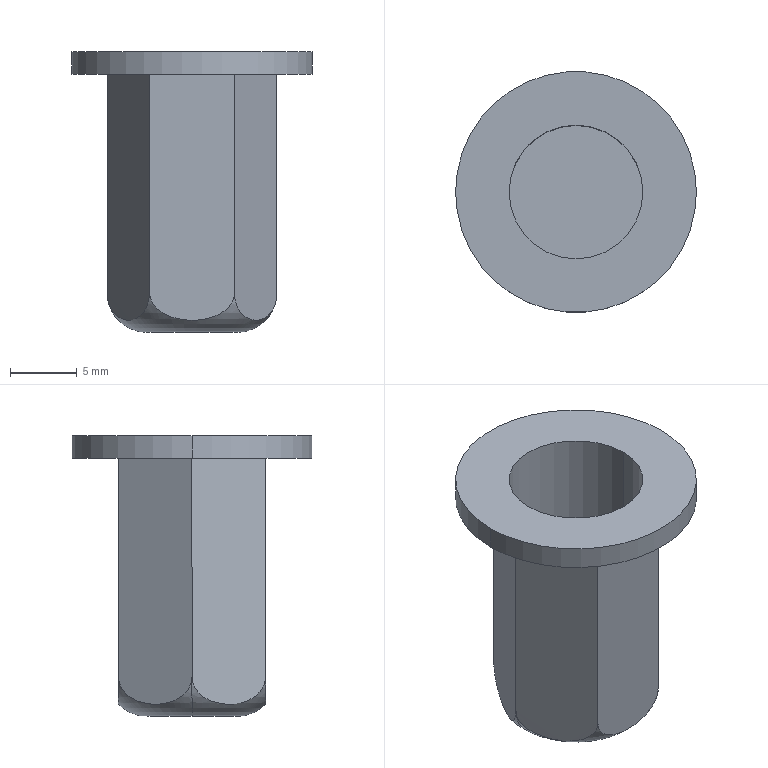Part | SolidWorks | features BaseBody 1 | 1 solid | 16 faces | box 18 x 18 x 21 mm | volume 1010 mm3 | plane 10 | cylinder 4 | torus 2 | commonest cylinder face diameters 10 x2 18 x2
STEP:
#1=CARTESIAN_POINT('',(5.,0.,-16.3));
#2=VERTEX_POINT('',#1);
#3=CARTESIAN_POINT('',(-5.,0.,-16.3));
#4=VERTEX_POINT('',#3);
#5=CARTESIAN_POINT('',(0.,0.,-16.3));
#6=DIRECTION('',(0.,0.,1.));
#7=DIRECTION('',(1.,0.,0.));
#8=AXIS2_PLACEMENT_3D('',#5,#6,#7);
#9=CIRCLE('',#8,5.);
#10=EDGE_CURVE('',#2,#4,#9,.T.);
#11=ORIENTED_EDGE('',*,*,#10,.T.);
#12=CARTESIAN_POINT('',(0.,0.,-16.3));
#13=DIRECTION('',(0.,0.,1.));
#14=DIRECTION('',(1.,0.,0.));
#15=AXIS2_PLACEMENT_3D('',#12,#13,#14);
#16=CIRCLE('',#15,5.);
#17=EDGE_CURVE('',#4,#2,#16,.T.);
#18=ORIENTED_EDGE('',*,*,#17,.T.);
#19=EDGE_LOOP('',(#11,#18));
#20=FACE_OUTER_BOUND('',#19,.T.);
#21=CARTESIAN_POINT('',(0.,0.,-16.3));
#22=DIRECTION('',(0.,0.,1.));
#23=DIRECTION('',(1.,0.,0.));
#24=AXIS2_PLACEMENT_3D('',#21,#22,#23);
#25=PLANE('',#24);
#26=ADVANCED_FACE('',(#20),#25,.T.);
#27=CARTESIAN_POINT('',(-5.,0.,1.7));
#28=VERTEX_POINT('',#27);
#29=CARTESIAN_POINT('',(-5.,0.,-16.3));
#30=DIRECTION('',(0.,0.,1.));
#31=VECTOR('',#30,1000.);
#32=LINE('',#29,#31);
#33=EDGE_CURVE('',#4,#28,#32,.T.);
#34=ORIENTED_EDGE('',*,*,#33,.F.);
#35=ORIENTED_EDGE('',*,*,#10,.F.);
#36=CARTESIAN_POINT('',(5.,0.,1.7));
#37=VERTEX_POINT('',#36);
#38=CARTESIAN_POINT('',(5.,0.,-16.3));
#39=DIRECTION('',(0.,0.,1.));
#40=VECTOR('',#39,1000.);
#41=LINE('',#38,#40);
#42=EDGE_CURVE('',#2,#37,#41,.T.);
#43=ORIENTED_EDGE('',*,*,#42,.T.);
#44=CARTESIAN_POINT('',(0.,0.,1.7));
#45=DIRECTION('',(0.,0.,1.));
#46=DIRECTION('',(1.,0.,0.));
#47=AXIS2_PLACEMENT_3D('',#44,#45,#46);
#48=CIRCLE('',#47,5.);
#49=EDGE_CURVE('',#37,#28,#48,.T.);
#50=ORIENTED_EDGE('',*,*,#49,.T.);
#51=EDGE_LOOP('',(#34,#35,#43,#50));
#52=FACE_OUTER_BOUND('',#51,.T.);
#53=CARTESIAN_POINT('',(0.,0.,-16.3));
#54=DIRECTION('',(0.,0.,1.));
#55=DIRECTION('',(1.,0.,0.));
#56=AXIS2_PLACEMENT_3D('',#53,#54,#55);
#57=CYLINDRICAL_SURFACE('',#56,5.);
#58=ADVANCED_FACE('',(#52),#57,.F.);
#59=CARTESIAN_POINT('',(3.351,0.,-19.3));
#60=VERTEX_POINT('',#59);
#61=CARTESIAN_POINT('',(-3.351,0.,-19.3));
#62=VERTEX_POINT('',#61);
#63=CARTESIAN_POINT('',(0.,0.,-19.3));
#64=DIRECTION('',(0.,0.,1.));
#65=DIRECTION('',(1.,0.,0.));
#66=AXIS2_PLACEMENT_3D('',#63,#64,#65);
#67=CIRCLE('',#66,3.351);
#68=EDGE_CURVE('',#60,#62,#67,.T.);
#69=ORIENTED_EDGE('',*,*,#68,.F.);
#70=CARTESIAN_POINT('',(0.,0.,-19.3));
#71=DIRECTION('',(0.,0.,1.));
#72=DIRECTION('',(1.,0.,0.));
#73=AXIS2_PLACEMENT_3D('',#70,#71,#72);
#74=CIRCLE('',#73,3.351);
#75=EDGE_CURVE('',#62,#60,#74,.T.);
#76=ORIENTED_EDGE('',*,*,#75,.F.);
#77=EDGE_LOOP('',(#69,#76));
#78=FACE_OUTER_BOUND('',#77,.T.);
#79=CARTESIAN_POINT('',(0.,0.,-19.3));
#80=DIRECTION('',(0.,0.,-1.));
#81=DIRECTION('',(0.,-1.,0.));
#82=AXIS2_PLACEMENT_3D('',#79,#80,#81);
#83=PLANE('',#82);
#84=ADVANCED_FACE('',(#78),#83,.T.);
#85=CARTESIAN_POINT('',(-6.351,0.,-16.3));
#86=VERTEX_POINT('',#85);
#87=CARTESIAN_POINT('',(-3.351,0.,-16.3));
#88=DIRECTION('',(0.,1.,0.));
#89=DIRECTION('',(-1.,0.,0.));
#90=AXIS2_PLACEMENT_3D('',#87,#88,#89);
#91=CIRCLE('',#90,3.);
#92=EDGE_CURVE('',#62,#86,#91,.T.);
#93=ORIENTED_EDGE('',*,*,#92,.F.);
#94=ORIENTED_EDGE('',*,*,#75,.T.);
#95=CARTESIAN_POINT('',(6.351,0.,-16.3));
#96=VERTEX_POINT('',#95);
#97=CARTESIAN_POINT('',(3.351,0.,-16.3));
#98=DIRECTION('',(0.,-1.,0.));
#99=DIRECTION('',(0.,0.,-1.));
#100=AXIS2_PLACEMENT_3D('',#97,#98,#99);
#101=CIRCLE('',#100,3.);
#102=EDGE_CURVE('',#60,#96,#101,.T.);
#103=ORIENTED_EDGE('',*,*,#102,.T.);
#104=CARTESIAN_POINT('',(3.175,-5.5,-16.3));
#105=VERTEX_POINT('',#104);
#106=CARTESIAN_POINT('',(6.351,0.,-16.3));
#107=CARTESIAN_POINT('',(6.351,0.,-16.389));
#108=CARTESIAN_POINT('',(6.347,-0.006559,-16.475));
#109=CARTESIAN_POINT('',(6.332,-0.03267,-16.647));
#110=CARTESIAN_POINT('',(6.321,-0.05223,-16.732));
#111=CARTESIAN_POINT('',(6.291,-0.1039,-16.899));
#112=CARTESIAN_POINT('',(6.273,-0.1343,-16.977));
#113=CARTESIAN_POINT('',(6.231,-0.2069,-17.131));
#114=CARTESIAN_POINT('',(6.207,-0.2487,-17.205));
#115=CARTESIAN_POINT('',(6.173,-0.3072,-17.295));
#116=CARTESIAN_POINT('',(6.167,-0.3179,-17.311));
#117=CARTESIAN_POINT('',(6.154,-0.341,-17.344));
#118=CARTESIAN_POINT('',(6.133,-0.3764,-17.393));
#119=CARTESIAN_POINT('',(6.112,-0.4138,-17.441));
#120=CARTESIAN_POINT('',(6.067,-0.4914,-17.533));
#121=CARTESIAN_POINT('',(6.035,-0.5466,-17.592));
#122=CARTESIAN_POINT('',(5.933,-0.7223,-17.757));
#123=CARTESIAN_POINT('',(5.859,-0.8527,-17.855));
#124=CARTESIAN_POINT('',(5.767,-1.012,-17.953));
#125=CARTESIAN_POINT('',(5.758,-1.027,-17.962));
#126=CARTESIAN_POINT('',(5.739,-1.06,-17.981));
#127=CARTESIAN_POINT('',(5.71,-1.11,-18.009));
#128=CARTESIAN_POINT('',(5.681,-1.161,-18.036));
#129=CARTESIAN_POINT('',(5.621,-1.263,-18.087));
#130=CARTESIAN_POINT('',(5.581,-1.333,-18.118));
#131=CARTESIAN_POINT('',(5.458,-1.546,-18.204));
#132=CARTESIAN_POINT('',(5.373,-1.694,-18.251));
#133=CARTESIAN_POINT('',(5.261,-1.887,-18.297));
#134=CARTESIAN_POINT('',(5.241,-1.922,-18.305));
#135=CARTESIAN_POINT('',(5.198,-1.996,-18.321));
#136=CARTESIAN_POINT('',(5.177,-2.033,-18.328));
#137=CARTESIAN_POINT('',(5.113,-2.144,-18.348));
#138=CARTESIAN_POINT('',(5.07,-2.218,-18.358));
#139=CARTESIAN_POINT('',(4.941,-2.442,-18.384));
#140=CARTESIAN_POINT('',(4.853,-2.594,-18.393));
#141=CARTESIAN_POINT('',(4.587,-3.056,-18.393));
#142=CARTESIAN_POINT('',(4.415,-3.354,-18.36));
#143=CARTESIAN_POINT('',(4.223,-3.686,-18.28));
#144=CARTESIAN_POINT('',(4.2,-3.726,-18.269));
#145=CARTESIAN_POINT('',(4.156,-3.801,-18.248));
#146=CARTESIAN_POINT('',(4.134,-3.839,-18.237));
#147=CARTESIAN_POINT('',(4.07,-3.95,-18.202));
#148=CARTESIAN_POINT('',(4.028,-4.023,-18.176));
#149=CARTESIAN_POINT('',(3.905,-4.236,-18.09));
#150=CARTESIAN_POINT('',(3.826,-4.373,-18.022));
#151=CARTESIAN_POINT('',(3.741,-4.521,-17.933));
#152=CARTESIAN_POINT('',(3.73,-4.539,-17.921));
#153=CARTESIAN_POINT('',(3.71,-4.574,-17.899));
#154=CARTESIAN_POINT('',(3.68,-4.625,-17.865));
#155=CARTESIAN_POINT('',(3.652,-4.675,-17.829));
#156=CARTESIAN_POINT('',(3.595,-4.772,-17.756));
#157=CARTESIAN_POINT('',(3.56,-4.834,-17.704));
#158=CARTESIAN_POINT('',(3.458,-5.01,-17.539));
#159=CARTESIAN_POINT('',(3.398,-5.114,-17.416));
#160=CARTESIAN_POINT('',(3.341,-5.214,-17.263));
#161=CARTESIAN_POINT('',(3.334,-5.226,-17.244));
#162=CARTESIAN_POINT('',(3.321,-5.248,-17.208));
#163=CARTESIAN_POINT('',(3.302,-5.28,-17.152));
#164=CARTESIAN_POINT('',(3.285,-5.31,-17.096));
#165=CARTESIAN_POINT('',(3.254,-5.364,-16.98));
#166=CARTESIAN_POINT('',(3.236,-5.395,-16.901));
#167=CARTESIAN_POINT('',(3.214,-5.434,-16.778));
#168=CARTESIAN_POINT('',(3.207,-5.445,-16.734));
#169=CARTESIAN_POINT('',(3.195,-5.465,-16.649));
#170=CARTESIAN_POINT('',(3.191,-5.473,-16.606));
#171=CARTESIAN_POINT('',(3.179,-5.493,-16.476));
#172=CARTESIAN_POINT('',(3.175,-5.5,-16.388));
#173=CARTESIAN_POINT('',(3.175,-5.5,-16.3));
#174=B_SPLINE_CURVE_WITH_KNOTS('',3,(#106,#107,#108,#109,#110,#111,#112,#113,#114,#115,#116,#117,#118,#119,#120,#121,#122,#123,#124,#125,#126,#127,#128,#129,#130,#131,#132,#133,#134,#135,#136,#137,#138,#139,#140,#141,#142,#143,#144,#145,#146,#147,#148,#149,#150,#151,#152,#153,#154,#155,#156,#157,#158,#159,#160,#161,#162,#163,#164,#165,#166,#167,#168,#169,#170,#171,#172,#173),.UNSPECIFIED.,.F.,.F.,(4,2,2,2,2,2,1,2,2,2,2,1,2,2,2,2,2,2,2,2,2,2,2,2,2,1,2,2,2,2,1,2,2,2,2,4),(0.,0.03125,0.0625,0.09375,0.125,0.1328,0.1406,0.1563,0.1875,0.25,0.2578,0.2656,0.2813,0.3125,0.375,0.3906,0.4063,0.4375,0.5,0.625,0.6406,0.6563,0.6875,0.75,0.7578,0.7656,0.7813,0.8125,0.875,0.8828,0.8906,0.9063,0.9375,0.9531,0.9688,1.),.UNSPECIFIED.);
#175=EDGE_CURVE('',#96,#105,#174,.T.);
#176=ORIENTED_EDGE('',*,*,#175,.T.);
#177=CARTESIAN_POINT('',(-3.175,-5.5,-16.3));
#178=VERTEX_POINT('',#177);
#179=CARTESIAN_POINT('',(3.175,-5.5,-16.3));
#180=CARTESIAN_POINT('',(3.175,-5.5,-16.388));
#181=CARTESIAN_POINT('',(3.168,-5.5,-16.475));
#182=CARTESIAN_POINT('',(3.145,-5.5,-16.605));
#183=CARTESIAN_POINT('',(3.136,-5.5,-16.647));
#184=CARTESIAN_POINT('',(3.113,-5.5,-16.733));
#185=CARTESIAN_POINT('',(3.099,-5.5,-16.776));
#186=CARTESIAN_POINT('',(3.055,-5.5,-16.899));
#187=CARTESIAN_POINT('',(3.02,-5.5,-16.978));
#188=CARTESIAN_POINT('',(2.957,-5.5,-17.094));
#189=CARTESIAN_POINT('',(2.923,-5.5,-17.151));
#190=CARTESIAN_POINT('',(2.885,-5.5,-17.206));
#191=CARTESIAN_POINT('',(2.86,-5.5,-17.243));
#192=CARTESIAN_POINT('',(2.846,-5.5,-17.262));
#193=CARTESIAN_POINT('',(2.731,-5.5,-17.415));
#194=CARTESIAN_POINT('',(2.61,-5.5,-17.537));
#195=CARTESIAN_POINT('',(2.408,-5.5,-17.703));
#196=CARTESIAN_POINT('',(2.336,-5.5,-17.755));
#197=CARTESIAN_POINT('',(2.224,-5.5,-17.828));
#198=CARTESIAN_POINT('',(2.167,-5.5,-17.864));
#199=CARTESIAN_POINT('',(2.107,-5.5,-17.898));
#200=CARTESIAN_POINT('',(2.067,-5.5,-17.92));
#201=CARTESIAN_POINT('',(2.045,-5.5,-17.932));
#202=CARTESIAN_POINT('',(1.876,-5.5,-18.022));
#203=CARTESIAN_POINT('',(1.718,-5.5,-18.09));
#204=CARTESIAN_POINT('',(1.472,-5.5,-18.175));
#205=CARTESIAN_POINT('',(1.388,-5.5,-18.201));
#206=CARTESIAN_POINT('',(1.26,-5.5,-18.236));
#207=CARTESIAN_POINT('',(1.217,-5.5,-18.248));
#208=CARTESIAN_POINT('',(1.13,-5.5,-18.269));
#209=CARTESIAN_POINT('',(1.084,-5.5,-18.279));
#210=CARTESIAN_POINT('',(0.8705,-5.5,-18.324));
#211=CARTESIAN_POINT('',(0.6987,-5.5,-18.35));
#212=CARTESIAN_POINT('',(0.3513,-5.5,-18.385));
#213=CARTESIAN_POINT('',(0.1745,-5.5,-18.393));
#214=CARTESIAN_POINT('',(-0.1812,-5.5,-18.393));
#215=CARTESIAN_POINT('',(-0.3557,-5.5,-18.384));
#216=CARTESIAN_POINT('',(-0.6145,-5.5,-18.358));
#217=CARTESIAN_POINT('',(-0.7003,-5.5,-18.348));
#218=CARTESIAN_POINT('',(-0.8286,-5.5,-18.328));
#219=CARTESIAN_POINT('',(-0.8713,-5.5,-18.321));
#220=CARTESIAN_POINT('',(-0.9565,-5.5,-18.305));
#221=CARTESIAN_POINT('',(-0.997,-5.5,-18.297));
#222=CARTESIAN_POINT('',(-1.22,-5.5,-18.25));
#223=CARTESIAN_POINT('',(-1.391,-5.5,-18.204));
#224=CARTESIAN_POINT('',(-1.638,-5.5,-18.118));
#225=CARTESIAN_POINT('',(-1.718,-5.5,-18.086));
#226=CARTESIAN_POINT('',(-1.837,-5.5,-18.035));
#227=CARTESIAN_POINT('',(-1.895,-5.5,-18.008));
#228=CARTESIAN_POINT('',(-1.953,-5.5,-17.98));
#229=CARTESIAN_POINT('',(-1.991,-5.5,-17.961));
#230=CARTESIAN_POINT('',(-2.009,-5.5,-17.952));
#231=CARTESIAN_POINT('',(-2.192,-5.5,-17.854));
#232=CARTESIAN_POINT('',(-2.342,-5.5,-17.756));
#233=CARTESIAN_POINT('',(-2.545,-5.5,-17.591));
#234=CARTESIAN_POINT('',(-2.609,-5.5,-17.533));
#235=CARTESIAN_POINT('',(-2.698,-5.5,-17.44));
#236=CARTESIAN_POINT('',(-2.741,-5.5,-17.393));
#237=CARTESIAN_POINT('',(-2.782,-5.5,-17.344));
#238=CARTESIAN_POINT('',(-2.809,-5.5,-17.31));
#239=CARTESIAN_POINT('',(-2.821,-5.5,-17.295));
#240=CARTESIAN_POINT('',(-2.888,-5.5,-17.205));
#241=CARTESIAN_POINT('',(-2.937,-5.5,-17.13));
#242=CARTESIAN_POINT('',(-3.02,-5.5,-16.977));
#243=CARTESIAN_POINT('',(-3.055,-5.5,-16.899));
#244=CARTESIAN_POINT('',(-3.145,-5.5,-16.648));
#245=CARTESIAN_POINT('',(-3.175,-5.5,-16.475));
#246=CARTESIAN_POINT('',(-3.175,-5.5,-16.3));
#247=B_SPLINE_CURVE_WITH_KNOTS('',3,(#179,#180,#181,#182,#183,#184,#185,#186,#187,#188,#189,#190,#191,#192,#193,#194,#195,#196,#197,#198,#199,#200,#201,#202,#203,#204,#205,#206,#207,#208,#209,#210,#211,#212,#213,#214,#215,#216,#217,#218,#219,#220,#221,#222,#223,#224,#225,#226,#227,#228,#229,#230,#231,#232,#233,#234,#235,#236,#237,#238,#239,#240,#241,#242,#243,#244,#245,#246),.UNSPECIFIED.,.F.,.F.,(4,2,2,2,2,1,2,2,2,2,1,2,2,2,2,2,2,2,2,2,2,2,2,2,2,1,2,2,2,2,1,2,2,2,2,4),(0.,0.03125,0.04688,0.0625,0.09375,0.1094,0.1172,0.125,0.1875,0.2188,0.2344,0.2422,0.25,0.3125,0.3438,0.3594,0.375,0.4375,0.5,0.5625,0.5938,0.6094,0.625,0.6875,0.7188,0.7344,0.7422,0.75,0.8125,0.8438,0.8594,0.8672,0.875,0.9063,0.9375,1.),.UNSPECIFIED.);
#248=EDGE_CURVE('',#105,#178,#247,.T.);
#249=ORIENTED_EDGE('',*,*,#248,.T.);
#250=CARTESIAN_POINT('',(-3.175,-5.5,-16.3));
#251=CARTESIAN_POINT('',(-3.175,-5.5,-16.388));
#252=CARTESIAN_POINT('',(-3.179,-5.493,-16.475));
#253=CARTESIAN_POINT('',(-3.194,-5.467,-16.647));
#254=CARTESIAN_POINT('',(-3.206,-5.447,-16.734));
#255=CARTESIAN_POINT('',(-3.235,-5.397,-16.897));
#256=CARTESIAN_POINT('',(-3.253,-5.366,-16.977));
#257=CARTESIAN_POINT('',(-3.284,-5.311,-17.092));
#258=CARTESIAN_POINT('',(-3.301,-5.282,-17.149));
#259=CARTESIAN_POINT('',(-3.32,-5.25,-17.204));
#260=CARTESIAN_POINT('',(-3.333,-5.228,-17.241));
#261=CARTESIAN_POINT('',(-3.34,-5.216,-17.26));
#262=CARTESIAN_POINT('',(-3.397,-5.116,-17.413));
#263=CARTESIAN_POINT('',(-3.457,-5.012,-17.536));
#264=CARTESIAN_POINT('',(-3.558,-4.836,-17.702));
#265=CARTESIAN_POINT('',(-3.594,-4.774,-17.754));
#266=CARTESIAN_POINT('',(-3.651,-4.677,-17.828));
#267=CARTESIAN_POINT('',(-3.679,-4.627,-17.864));
#268=CARTESIAN_POINT('',(-3.709,-4.576,-17.898));
#269=CARTESIAN_POINT('',(-3.729,-4.541,-17.92));
#270=CARTESIAN_POINT('',(-3.74,-4.522,-17.932));
#271=CARTESIAN_POINT('',(-3.825,-4.375,-18.022));
#272=CARTESIAN_POINT('',(-3.904,-4.238,-18.089));
#273=CARTESIAN_POINT('',(-4.027,-4.025,-18.175));
#274=CARTESIAN_POINT('',(-4.069,-3.952,-18.201));
#275=CARTESIAN_POINT('',(-4.133,-3.841,-18.236));
#276=CARTESIAN_POINT('',(-4.155,-3.804,-18.248));
#277=CARTESIAN_POINT('',(-4.198,-3.728,-18.269));
#278=CARTESIAN_POINT('',(-4.221,-3.688,-18.279));
#279=CARTESIAN_POINT('',(-4.413,-3.357,-18.359));
#280=CARTESIAN_POINT('',(-4.583,-3.061,-18.393));
#281=CARTESIAN_POINT('',(-4.851,-2.598,-18.393));
#282=CARTESIAN_POINT('',(-4.938,-2.446,-18.385));
#283=CARTESIAN_POINT('',(-5.068,-2.222,-18.359));
#284=CARTESIAN_POINT('',(-5.111,-2.147,-18.348));
#285=CARTESIAN_POINT('',(-5.175,-2.036,-18.328));
#286=CARTESIAN_POINT('',(-5.197,-1.999,-18.321));
#287=CARTESIAN_POINT('',(-5.24,-1.925,-18.306));
#288=CARTESIAN_POINT('',(-5.26,-1.889,-18.298));
#289=CARTESIAN_POINT('',(-5.371,-1.697,-18.251));
#290=CARTESIAN_POINT('',(-5.457,-1.548,-18.205));
#291=CARTESIAN_POINT('',(-5.58,-1.335,-18.119));
#292=CARTESIAN_POINT('',(-5.62,-1.265,-18.088));
#293=CARTESIAN_POINT('',(-5.68,-1.162,-18.037));
#294=CARTESIAN_POINT('',(-5.709,-1.112,-18.01));
#295=CARTESIAN_POINT('',(-5.738,-1.062,-17.982));
#296=CARTESIAN_POINT('',(-5.757,-1.029,-17.962));
#297=CARTESIAN_POINT('',(-5.766,-1.013,-17.953));
#298=CARTESIAN_POINT('',(-5.858,-0.8544,-17.856));
#299=CARTESIAN_POINT('',(-5.932,-0.7243,-17.759));
#300=CARTESIAN_POINT('',(-6.034,-0.5487,-17.594));
#301=CARTESIAN_POINT('',(-6.066,-0.4935,-17.535));
#302=CARTESIAN_POINT('',(-6.111,-0.4159,-17.443));
#303=CARTESIAN_POINT('',(-6.132,-0.3785,-17.396));
#304=CARTESIAN_POINT('',(-6.153,-0.3431,-17.347));
#305=CARTESIAN_POINT('',(-6.166,-0.32,-17.314));
#306=CARTESIAN_POINT('',(-6.172,-0.3093,-17.298));
#307=CARTESIAN_POINT('',(-6.206,-0.2506,-17.208));
#308=CARTESIAN_POINT('',(-6.23,-0.2087,-17.134));
#309=CARTESIAN_POINT('',(-6.262,-0.154,-17.019));
#310=CARTESIAN_POINT('',(-6.272,-0.1371,-16.98));
#311=CARTESIAN_POINT('',(-6.29,-0.106,-16.9));
#312=CARTESIAN_POINT('',(-6.298,-0.09231,-16.861));
#313=CARTESIAN_POINT('',(-6.335,-0.02678,-16.65));
#314=CARTESIAN_POINT('',(-6.351,0.,-16.477));
#315=CARTESIAN_POINT('',(-6.351,0.,-16.3));
#316=B_SPLINE_CURVE_WITH_KNOTS('',3,(#250,#251,#252,#253,#254,#255,#256,#257,#258,#259,#260,#261,#262,#263,#264,#265,#266,#267,#268,#269,#270,#271,#272,#273,#274,#275,#276,#277,#278,#279,#280,#281,#282,#283,#284,#285,#286,#287,#288,#289,#290,#291,#292,#293,#294,#295,#296,#297,#298,#299,#300,#301,#302,#303,#304,#305,#306,#307,#308,#309,#310,#311,#312,#313,#314,#315),.UNSPECIFIED.,.F.,.F.,(4,2,2,2,1,2,2,2,2,1,2,2,2,2,2,2,2,2,2,2,2,2,2,1,2,2,2,2,1,2,2,2,2,2,4),(0.,0.03125,0.0625,0.09375,0.1094,0.1172,0.125,0.1875,0.2188,0.2344,0.2422,0.25,0.3125,0.3438,0.3594,0.375,0.5,0.5625,0.5938,0.6094,0.625,0.6875,0.7188,0.7344,0.7422,0.75,0.8125,0.8438,0.8594,0.8672,0.875,0.9063,0.9219,0.9375,1.),.UNSPECIFIED.);
#317=EDGE_CURVE('',#178,#86,#316,.T.);
#318=ORIENTED_EDGE('',*,*,#317,.T.);
#319=EDGE_LOOP('',(#93,#94,#103,#176,#249,#318));
#320=FACE_OUTER_BOUND('',#319,.T.);
#321=CARTESIAN_POINT('',(0.,0.,-16.3));
#322=DIRECTION('',(0.,0.,1.));
#323=DIRECTION('',(1.,0.,0.));
#324=AXIS2_PLACEMENT_3D('',#321,#322,#323);
#325=TOROIDAL_SURFACE('',#324,3.351,3.);
#326=ADVANCED_FACE('',(#320),#325,.T.);
#327=ORIENTED_EDGE('',*,*,#49,.F.);
#328=CARTESIAN_POINT('',(0.,0.,1.7));
#329=DIRECTION('',(0.,0.,1.));
#330=DIRECTION('',(1.,0.,0.));
#331=AXIS2_PLACEMENT_3D('',#328,#329,#330);
#332=CIRCLE('',#331,5.);
#333=EDGE_CURVE('',#28,#37,#332,.T.);
#334=ORIENTED_EDGE('',*,*,#333,.F.);
#335=EDGE_LOOP('',(#327,#334));
#336=FACE_BOUND('',#335,.T.);
#337=CARTESIAN_POINT('',(-9.,0.,1.7));
#338=VERTEX_POINT('',#337);
#339=CARTESIAN_POINT('',(9.,0.,1.7));
#340=VERTEX_POINT('',#339);
#341=CARTESIAN_POINT('',(0.,0.,1.7));
#342=DIRECTION('',(0.,0.,1.));
#343=DIRECTION('',(1.,0.,0.));
#344=AXIS2_PLACEMENT_3D('',#341,#342,#343);
#345=CIRCLE('',#344,9.);
#346=EDGE_CURVE('',#338,#340,#345,.T.);
#347=ORIENTED_EDGE('',*,*,#346,.T.);
#348=CARTESIAN_POINT('',(0.,0.,1.7));
#349=DIRECTION('',(0.,0.,1.));
#350=DIRECTION('',(1.,0.,0.));
#351=AXIS2_PLACEMENT_3D('',#348,#349,#350);
#352=CIRCLE('',#351,9.);
#353=EDGE_CURVE('',#340,#338,#352,.T.);
#354=ORIENTED_EDGE('',*,*,#353,.T.);
#355=EDGE_LOOP('',(#347,#354));
#356=FACE_OUTER_BOUND('',#355,.T.);
#357=CARTESIAN_POINT('',(0.,0.,1.7));
#358=DIRECTION('',(0.,0.,1.));
#359=DIRECTION('',(1.,0.,0.));
#360=AXIS2_PLACEMENT_3D('',#357,#358,#359);
#361=PLANE('',#360);
#362=ADVANCED_FACE('',(#336,#356),#361,.T.);
#363=CARTESIAN_POINT('',(9.,0.,0.));
#364=VERTEX_POINT('',#363);
#365=CARTESIAN_POINT('',(9.,0.,1.7));
#366=DIRECTION('',(0.,0.,-1.));
#367=VECTOR('',#366,1000.);
#368=LINE('',#365,#367);
#369=EDGE_CURVE('',#340,#364,#368,.T.);
#370=ORIENTED_EDGE('',*,*,#369,.F.);
#371=ORIENTED_EDGE('',*,*,#346,.F.);
#372=CARTESIAN_POINT('',(-9.,0.,0.));
#373=VERTEX_POINT('',#372);
#374=CARTESIAN_POINT('',(-9.,0.,1.7));
#375=DIRECTION('',(0.,0.,-1.));
#376=VECTOR('',#375,1000.);
#377=LINE('',#374,#376);
#378=EDGE_CURVE('',#338,#373,#377,.T.);
#379=ORIENTED_EDGE('',*,*,#378,.T.);
#380=CARTESIAN_POINT('',(0.,0.,0.));
#381=DIRECTION('',(0.,0.,1.));
#382=DIRECTION('',(1.,0.,0.));
#383=AXIS2_PLACEMENT_3D('',#380,#381,#382);
#384=CIRCLE('',#383,9.);
#385=EDGE_CURVE('',#373,#364,#384,.T.);
#386=ORIENTED_EDGE('',*,*,#385,.T.);
#387=EDGE_LOOP('',(#370,#371,#379,#386));
#388=FACE_OUTER_BOUND('',#387,.T.);
#389=CARTESIAN_POINT('',(0.,0.,1.7));
#390=DIRECTION('',(0.,0.,-1.));
#391=DIRECTION('',(-1.,0.,0.));
#392=AXIS2_PLACEMENT_3D('',#389,#390,#391);
#393=CYLINDRICAL_SURFACE('',#392,9.);
#394=ADVANCED_FACE('',(#388),#393,.T.);
#395=CARTESIAN_POINT('',(-3.175,-5.5,0.));
#396=VERTEX_POINT('',#395);
#397=CARTESIAN_POINT('',(-6.351,0.,0.));
#398=VERTEX_POINT('',#397);
#399=CARTESIAN_POINT('',(-3.175,-5.5,0.));
#400=DIRECTION('',(-0.5,0.866,0.));
#401=VECTOR('',#400,1000.);
#402=LINE('',#399,#401);
#403=EDGE_CURVE('',#396,#398,#402,.T.);
#404=ORIENTED_EDGE('',*,*,#403,.F.);
#405=CARTESIAN_POINT('',(3.175,-5.5,0.));
#406=VERTEX_POINT('',#405);
#407=CARTESIAN_POINT('',(3.175,-5.5,0.));
#408=DIRECTION('',(-1.,0.,0.));
#409=VECTOR('',#408,1000.);
#410=LINE('',#407,#409);
#411=EDGE_CURVE('',#406,#396,#410,.T.);
#412=ORIENTED_EDGE('',*,*,#411,.F.);
#413=CARTESIAN_POINT('',(6.351,0.,0.));
#414=VERTEX_POINT('',#413);
#415=CARTESIAN_POINT('',(6.351,0.,0.));
#416=DIRECTION('',(-0.5,-0.866,0.));
#417=VECTOR('',#416,1000.);
#418=LINE('',#415,#417);
#419=EDGE_CURVE('',#414,#406,#418,.T.);
#420=ORIENTED_EDGE('',*,*,#419,.F.);
#421=CARTESIAN_POINT('',(3.175,5.5,0.));
#422=VERTEX_POINT('',#421);
#423=CARTESIAN_POINT('',(3.175,5.5,0.));
#424=DIRECTION('',(0.5,-0.866,0.));
#425=VECTOR('',#424,1000.);
#426=LINE('',#423,#425);
#427=EDGE_CURVE('',#422,#414,#426,.T.);
#428=ORIENTED_EDGE('',*,*,#427,.F.);
#429=CARTESIAN_POINT('',(-3.175,5.5,0.));
#430=VERTEX_POINT('',#429);
#431=CARTESIAN_POINT('',(-3.175,5.5,0.));
#432=DIRECTION('',(1.,0.,0.));
#433=VECTOR('',#432,1000.);
#434=LINE('',#431,#433);
#435=EDGE_CURVE('',#430,#422,#434,.T.);
#436=ORIENTED_EDGE('',*,*,#435,.F.);
#437=CARTESIAN_POINT('',(-6.351,0.,0.));
#438=DIRECTION('',(0.5,0.866,0.));
#439=VECTOR('',#438,1000.);
#440=LINE('',#437,#439);
#441=EDGE_CURVE('',#398,#430,#440,.T.);
#442=ORIENTED_EDGE('',*,*,#441,.F.);
#443=EDGE_LOOP('',(#404,#412,#420,#428,#436,#442));
#444=FACE_BOUND('',#443,.T.);
#445=ORIENTED_EDGE('',*,*,#385,.F.);
#446=CARTESIAN_POINT('',(0.,0.,0.));
#447=DIRECTION('',(0.,0.,1.));
#448=DIRECTION('',(1.,0.,0.));
#449=AXIS2_PLACEMENT_3D('',#446,#447,#448);
#450=CIRCLE('',#449,9.);
#451=EDGE_CURVE('',#364,#373,#450,.T.);
#452=ORIENTED_EDGE('',*,*,#451,.F.);
#453=EDGE_LOOP('',(#445,#452));
#454=FACE_OUTER_BOUND('',#453,.T.);
#455=CARTESIAN_POINT('',(0.,0.,0.));
#456=DIRECTION('',(0.,0.,1.));
#457=DIRECTION('',(1.,0.,0.));
#458=AXIS2_PLACEMENT_3D('',#455,#456,#457);
#459=PLANE('',#458);
#460=ADVANCED_FACE('',(#444,#454),#459,.F.);
#461=ORIENTED_EDGE('',*,*,#248,.F.);
#462=CARTESIAN_POINT('',(3.175,-5.5,-19.3));
#463=DIRECTION('',(0.,0.,1.));
#464=VECTOR('',#463,1000.);
#465=LINE('',#462,#464);
#466=EDGE_CURVE('',#105,#406,#465,.T.);
#467=ORIENTED_EDGE('',*,*,#466,.T.);
#468=ORIENTED_EDGE('',*,*,#411,.T.);
#469=CARTESIAN_POINT('',(-3.175,-5.5,-19.3));
#470=DIRECTION('',(0.,0.,1.));
#471=VECTOR('',#470,1000.);
#472=LINE('',#469,#471);
#473=EDGE_CURVE('',#178,#396,#472,.T.);
#474=ORIENTED_EDGE('',*,*,#473,.F.);
#475=EDGE_LOOP('',(#461,#467,#468,#474));
#476=FACE_OUTER_BOUND('',#475,.T.);
#477=CARTESIAN_POINT('',(3.175,-5.5,-19.3));
#478=DIRECTION('',(0.,1.,0.));
#479=DIRECTION('',(1.,0.,0.));
#480=AXIS2_PLACEMENT_3D('',#477,#478,#479);
#481=PLANE('',#480);
#482=ADVANCED_FACE('',(#476),#481,.F.);
#483=ORIENTED_EDGE('',*,*,#175,.F.);
#484=CARTESIAN_POINT('',(6.351,0.,-19.3));
#485=DIRECTION('',(0.,0.,1.));
#486=VECTOR('',#485,1000.);
#487=LINE('',#484,#486);
#488=EDGE_CURVE('',#96,#414,#487,.T.);
#489=ORIENTED_EDGE('',*,*,#488,.T.);
#490=ORIENTED_EDGE('',*,*,#419,.T.);
#491=ORIENTED_EDGE('',*,*,#466,.F.);
#492=EDGE_LOOP('',(#483,#489,#490,#491));
#493=FACE_OUTER_BOUND('',#492,.T.);
#494=CARTESIAN_POINT('',(6.351,0.,-19.3));
#495=DIRECTION('',(-0.866,0.5,0.));
#496=DIRECTION('',(0.,0.,1.));
#497=AXIS2_PLACEMENT_3D('',#494,#495,#496);
#498=PLANE('',#497);
#499=ADVANCED_FACE('',(#493),#498,.F.);
#500=CARTESIAN_POINT('',(3.175,5.5,-16.3));
#501=VERTEX_POINT('',#500);
#502=CARTESIAN_POINT('',(3.175,5.5,-16.3));
#503=CARTESIAN_POINT('',(3.175,5.5,-16.388));
#504=CARTESIAN_POINT('',(3.179,5.493,-16.475));
#505=CARTESIAN_POINT('',(3.194,5.467,-16.647));
#506=CARTESIAN_POINT('',(3.206,5.447,-16.734));
#507=CARTESIAN_POINT('',(3.235,5.397,-16.897));
#508=CARTESIAN_POINT('',(3.253,5.366,-16.977));
#509=CARTESIAN_POINT('',(3.284,5.311,-17.092));
#510=CARTESIAN_POINT('',(3.301,5.282,-17.149));
#511=CARTESIAN_POINT('',(3.32,5.25,-17.204));
#512=CARTESIAN_POINT('',(3.333,5.228,-17.241));
#513=CARTESIAN_POINT('',(3.34,5.216,-17.26));
#514=CARTESIAN_POINT('',(3.397,5.116,-17.413));
#515=CARTESIAN_POINT('',(3.457,5.012,-17.536));
#516=CARTESIAN_POINT('',(3.558,4.836,-17.702));
#517=CARTESIAN_POINT('',(3.594,4.774,-17.754));
#518=CARTESIAN_POINT('',(3.651,4.677,-17.828));
#519=CARTESIAN_POINT('',(3.679,4.627,-17.864));
#520=CARTESIAN_POINT('',(3.709,4.576,-17.898));
#521=CARTESIAN_POINT('',(3.729,4.541,-17.92));
#522=CARTESIAN_POINT('',(3.74,4.522,-17.932));
#523=CARTESIAN_POINT('',(3.825,4.375,-18.022));
#524=CARTESIAN_POINT('',(3.904,4.238,-18.089));
#525=CARTESIAN_POINT('',(4.027,4.025,-18.175));
#526=CARTESIAN_POINT('',(4.069,3.952,-18.201));
#527=CARTESIAN_POINT('',(4.133,3.841,-18.236));
#528=CARTESIAN_POINT('',(4.155,3.804,-18.248));
#529=CARTESIAN_POINT('',(4.198,3.728,-18.269));
#530=CARTESIAN_POINT('',(4.221,3.688,-18.279));
#531=CARTESIAN_POINT('',(4.413,3.357,-18.359));
#532=CARTESIAN_POINT('',(4.583,3.061,-18.393));
#533=CARTESIAN_POINT('',(4.851,2.598,-18.393));
#534=CARTESIAN_POINT('',(4.938,2.446,-18.385));
#535=CARTESIAN_POINT('',(5.068,2.222,-18.359));
#536=CARTESIAN_POINT('',(5.111,2.147,-18.348));
#537=CARTESIAN_POINT('',(5.175,2.036,-18.328));
#538=CARTESIAN_POINT('',(5.197,1.999,-18.321));
#539=CARTESIAN_POINT('',(5.24,1.925,-18.306));
#540=CARTESIAN_POINT('',(5.26,1.889,-18.298));
#541=CARTESIAN_POINT('',(5.371,1.697,-18.251));
#542=CARTESIAN_POINT('',(5.457,1.548,-18.205));
#543=CARTESIAN_POINT('',(5.58,1.335,-18.119));
#544=CARTESIAN_POINT('',(5.62,1.265,-18.088));
#545=CARTESIAN_POINT('',(5.68,1.162,-18.037));
#546=CARTESIAN_POINT('',(5.709,1.112,-18.01));
#547=CARTESIAN_POINT('',(5.738,1.062,-17.982));
#548=CARTESIAN_POINT('',(5.757,1.029,-17.962));
#549=CARTESIAN_POINT('',(5.766,1.013,-17.953));
#550=CARTESIAN_POINT('',(5.858,0.8544,-17.856));
#551=CARTESIAN_POINT('',(5.932,0.7243,-17.759));
#552=CARTESIAN_POINT('',(6.034,0.5488,-17.594));
#553=CARTESIAN_POINT('',(6.066,0.4935,-17.535));
#554=CARTESIAN_POINT('',(6.111,0.416,-17.443));
#555=CARTESIAN_POINT('',(6.125,0.391,-17.412));
#556=CARTESIAN_POINT('',(6.153,0.3429,-17.347));
#557=CARTESIAN_POINT('',(6.166,0.321,-17.316));
#558=CARTESIAN_POINT('',(6.206,0.2506,-17.208));
#559=CARTESIAN_POINT('',(6.23,0.2087,-17.134));
#560=CARTESIAN_POINT('',(6.262,0.154,-17.019));
#561=CARTESIAN_POINT('',(6.272,0.1371,-16.98));
#562=CARTESIAN_POINT('',(6.29,0.1061,-16.9));
#563=CARTESIAN_POINT('',(6.298,0.09227,-16.861));
#564=CARTESIAN_POINT('',(6.335,0.02678,-16.65));
#565=CARTESIAN_POINT('',(6.351,-0.0006071,-16.478));
#566=CARTESIAN_POINT('',(6.351,0.,-16.3));
#567=B_SPLINE_CURVE_WITH_KNOTS('',3,(#502,#503,#504,#505,#506,#507,#508,#509,#510,#511,#512,#513,#514,#515,#516,#517,#518,#519,#520,#521,#522,#523,#524,#525,#526,#527,#528,#529,#530,#531,#532,#533,#534,#535,#536,#537,#538,#539,#540,#541,#542,#543,#544,#545,#546,#547,#548,#549,#550,#551,#552,#553,#554,#555,#556,#557,#558,#559,#560,#561,#562,#563,#564,#565,#566),.UNSPECIFIED.,.F.,.F.,(4,2,2,2,1,2,2,2,2,1,2,2,2,2,2,2,2,2,2,2,2,2,2,1,2,2,2,2,2,2,2,2,2,4),(0.,0.03125,0.0625,0.09375,0.1094,0.1172,0.125,0.1875,0.2188,0.2344,0.2422,0.25,0.3125,0.3438,0.3594,0.375,0.5,0.5625,0.5938,0.6094,0.625,0.6875,0.7188,0.7344,0.7422,0.75,0.8125,0.8438,0.8594,0.875,0.9062,0.9219,0.9375,1.),.UNSPECIFIED.);
#568=EDGE_CURVE('',#501,#96,#567,.T.);
#569=ORIENTED_EDGE('',*,*,#568,.F.);
#570=CARTESIAN_POINT('',(3.175,5.5,-19.3));
#571=DIRECTION('',(0.,0.,1.));
#572=VECTOR('',#571,1000.);
#573=LINE('',#570,#572);
#574=EDGE_CURVE('',#501,#422,#573,.T.);
#575=ORIENTED_EDGE('',*,*,#574,.T.);
#576=ORIENTED_EDGE('',*,*,#427,.T.);
#577=ORIENTED_EDGE('',*,*,#488,.F.);
#578=EDGE_LOOP('',(#569,#575,#576,#577));
#579=FACE_OUTER_BOUND('',#578,.T.);
#580=CARTESIAN_POINT('',(3.175,5.5,-19.3));
#581=DIRECTION('',(-0.866,-0.5,0.));
#582=DIRECTION('',(-0.5,0.866,0.));
#583=AXIS2_PLACEMENT_3D('',#580,#581,#582);
#584=PLANE('',#583);
#585=ADVANCED_FACE('',(#579),#584,.F.);
#586=CARTESIAN_POINT('',(-3.175,5.5,-16.3));
#587=VERTEX_POINT('',#586);
#588=CARTESIAN_POINT('',(-3.175,5.5,-16.3));
#589=CARTESIAN_POINT('',(-3.175,5.5,-16.388));
#590=CARTESIAN_POINT('',(-3.168,5.5,-16.475));
#591=CARTESIAN_POINT('',(-3.145,5.5,-16.605));
#592=CARTESIAN_POINT('',(-3.136,5.5,-16.647));
#593=CARTESIAN_POINT('',(-3.113,5.5,-16.733));
#594=CARTESIAN_POINT('',(-3.099,5.5,-16.776));
#595=CARTESIAN_POINT('',(-3.055,5.5,-16.899));
#596=CARTESIAN_POINT('',(-3.02,5.5,-16.978));
#597=CARTESIAN_POINT('',(-2.957,5.5,-17.094));
#598=CARTESIAN_POINT('',(-2.923,5.5,-17.151));
#599=CARTESIAN_POINT('',(-2.885,5.5,-17.206));
#600=CARTESIAN_POINT('',(-2.86,5.5,-17.243));
#601=CARTESIAN_POINT('',(-2.846,5.5,-17.262));
#602=CARTESIAN_POINT('',(-2.731,5.5,-17.415));
#603=CARTESIAN_POINT('',(-2.61,5.5,-17.537));
#604=CARTESIAN_POINT('',(-2.408,5.5,-17.703));
#605=CARTESIAN_POINT('',(-2.336,5.5,-17.755));
#606=CARTESIAN_POINT('',(-2.224,5.5,-17.828));
#607=CARTESIAN_POINT('',(-2.167,5.5,-17.864));
#608=CARTESIAN_POINT('',(-2.107,5.5,-17.898));
#609=CARTESIAN_POINT('',(-2.067,5.5,-17.92));
#610=CARTESIAN_POINT('',(-2.045,5.5,-17.932));
#611=CARTESIAN_POINT('',(-1.876,5.5,-18.022));
#612=CARTESIAN_POINT('',(-1.718,5.5,-18.09));
#613=CARTESIAN_POINT('',(-1.472,5.5,-18.175));
#614=CARTESIAN_POINT('',(-1.388,5.5,-18.201));
#615=CARTESIAN_POINT('',(-1.26,5.5,-18.236));
#616=CARTESIAN_POINT('',(-1.217,5.5,-18.248));
#617=CARTESIAN_POINT('',(-1.13,5.5,-18.269));
#618=CARTESIAN_POINT('',(-1.084,5.5,-18.279));
#619=CARTESIAN_POINT('',(-0.8705,5.5,-18.324));
#620=CARTESIAN_POINT('',(-0.6987,5.5,-18.35));
#621=CARTESIAN_POINT('',(-0.3513,5.5,-18.385));
#622=CARTESIAN_POINT('',(-0.1745,5.5,-18.393));
#623=CARTESIAN_POINT('',(0.1812,5.5,-18.393));
#624=CARTESIAN_POINT('',(0.3557,5.5,-18.384));
#625=CARTESIAN_POINT('',(0.6145,5.5,-18.358));
#626=CARTESIAN_POINT('',(0.7003,5.5,-18.348));
#627=CARTESIAN_POINT('',(0.8286,5.5,-18.328));
#628=CARTESIAN_POINT('',(0.8713,5.5,-18.321));
#629=CARTESIAN_POINT('',(0.9565,5.5,-18.305));
#630=CARTESIAN_POINT('',(0.997,5.5,-18.297));
#631=CARTESIAN_POINT('',(1.22,5.5,-18.25));
#632=CARTESIAN_POINT('',(1.391,5.5,-18.204));
#633=CARTESIAN_POINT('',(1.638,5.5,-18.118));
#634=CARTESIAN_POINT('',(1.718,5.5,-18.086));
#635=CARTESIAN_POINT('',(1.837,5.5,-18.035));
#636=CARTESIAN_POINT('',(1.895,5.5,-18.008));
#637=CARTESIAN_POINT('',(1.953,5.5,-17.98));
#638=CARTESIAN_POINT('',(1.991,5.5,-17.961));
#639=CARTESIAN_POINT('',(2.009,5.5,-17.952));
#640=CARTESIAN_POINT('',(2.192,5.5,-17.854));
#641=CARTESIAN_POINT('',(2.342,5.5,-17.756));
#642=CARTESIAN_POINT('',(2.545,5.5,-17.591));
#643=CARTESIAN_POINT('',(2.609,5.5,-17.533));
#644=CARTESIAN_POINT('',(2.698,5.5,-17.44));
#645=CARTESIAN_POINT('',(2.741,5.5,-17.393));
#646=CARTESIAN_POINT('',(2.782,5.5,-17.344));
#647=CARTESIAN_POINT('',(2.809,5.5,-17.31));
#648=CARTESIAN_POINT('',(2.821,5.5,-17.295));
#649=CARTESIAN_POINT('',(2.888,5.5,-17.205));
#650=CARTESIAN_POINT('',(2.937,5.5,-17.13));
#651=CARTESIAN_POINT('',(3.02,5.5,-16.977));
#652=CARTESIAN_POINT('',(3.055,5.5,-16.899));
#653=CARTESIAN_POINT('',(3.145,5.5,-16.648));
#654=CARTESIAN_POINT('',(3.175,5.5,-16.475));
#655=CARTESIAN_POINT('',(3.175,5.5,-16.3));
#656=B_SPLINE_CURVE_WITH_KNOTS('',3,(#588,#589,#590,#591,#592,#593,#594,#595,#596,#597,#598,#599,#600,#601,#602,#603,#604,#605,#606,#607,#608,#609,#610,#611,#612,#613,#614,#615,#616,#617,#618,#619,#620,#621,#622,#623,#624,#625,#626,#627,#628,#629,#630,#631,#632,#633,#634,#635,#636,#637,#638,#639,#640,#641,#642,#643,#644,#645,#646,#647,#648,#649,#650,#651,#652,#653,#654,#655),.UNSPECIFIED.,.F.,.F.,(4,2,2,2,2,1,2,2,2,2,1,2,2,2,2,2,2,2,2,2,2,2,2,2,2,1,2,2,2,2,1,2,2,2,2,4),(0.,0.03125,0.04688,0.0625,0.09375,0.1094,0.1172,0.125,0.1875,0.2187,0.2344,0.2422,0.25,0.3125,0.3437,0.3594,0.375,0.4375,0.5,0.5625,0.5938,0.6094,0.625,0.6875,0.7188,0.7344,0.7422,0.75,0.8125,0.8438,0.8594,0.8672,0.875,0.9063,0.9375,1.),.UNSPECIFIED.);
#657=EDGE_CURVE('',#587,#501,#656,.T.);
#658=ORIENTED_EDGE('',*,*,#657,.F.);
#659=CARTESIAN_POINT('',(-3.175,5.5,-19.3));
#660=DIRECTION('',(0.,0.,1.));
#661=VECTOR('',#660,1000.);
#662=LINE('',#659,#661);
#663=EDGE_CURVE('',#587,#430,#662,.T.);
#664=ORIENTED_EDGE('',*,*,#663,.T.);
#665=ORIENTED_EDGE('',*,*,#435,.T.);
#666=ORIENTED_EDGE('',*,*,#574,.F.);
#667=EDGE_LOOP('',(#658,#664,#665,#666));
#668=FACE_OUTER_BOUND('',#667,.T.);
#669=CARTESIAN_POINT('',(-3.175,5.5,-19.3));
#670=DIRECTION('',(0.,-1.,0.));
#671=DIRECTION('',(0.,0.,-1.));
#672=AXIS2_PLACEMENT_3D('',#669,#670,#671);
#673=PLANE('',#672);
#674=ADVANCED_FACE('',(#668),#673,.F.);
#675=CARTESIAN_POINT('',(-6.351,0.,-16.3));
#676=CARTESIAN_POINT('',(-6.351,0.,-16.388));
#677=CARTESIAN_POINT('',(-6.347,0.006564,-16.475));
#678=CARTESIAN_POINT('',(-6.332,0.03268,-16.647));
#679=CARTESIAN_POINT('',(-6.32,0.05283,-16.734));
#680=CARTESIAN_POINT('',(-6.291,0.1033,-16.897));
#681=CARTESIAN_POINT('',(-6.273,0.1343,-16.977));
#682=CARTESIAN_POINT('',(-6.242,0.1888,-17.092));
#683=CARTESIAN_POINT('',(-6.225,0.218,-17.149));
#684=CARTESIAN_POINT('',(-6.206,0.2503,-17.204));
#685=CARTESIAN_POINT('',(-6.194,0.2724,-17.241));
#686=CARTESIAN_POINT('',(-6.187,0.2844,-17.26));
#687=CARTESIAN_POINT('',(-6.129,0.3842,-17.413));
#688=CARTESIAN_POINT('',(-6.069,0.4881,-17.536));
#689=CARTESIAN_POINT('',(-5.967,0.6638,-17.702));
#690=CARTESIAN_POINT('',(-5.932,0.7256,-17.754));
#691=CARTESIAN_POINT('',(-5.876,0.823,-17.828));
#692=CARTESIAN_POINT('',(-5.847,0.8729,-17.864));
#693=CARTESIAN_POINT('',(-5.817,0.9244,-17.898));
#694=CARTESIAN_POINT('',(-5.797,0.9591,-17.92));
#695=CARTESIAN_POINT('',(-5.786,0.978,-17.932));
#696=CARTESIAN_POINT('',(-5.701,1.125,-18.022));
#697=CARTESIAN_POINT('',(-5.622,1.262,-18.089));
#698=CARTESIAN_POINT('',(-5.499,1.475,-18.175));
#699=CARTESIAN_POINT('',(-5.457,1.548,-18.201));
#700=CARTESIAN_POINT('',(-5.393,1.659,-18.236));
#701=CARTESIAN_POINT('',(-5.371,1.696,-18.248));
#702=CARTESIAN_POINT('',(-5.328,1.772,-18.269));
#703=CARTESIAN_POINT('',(-5.305,1.812,-18.279));
#704=CARTESIAN_POINT('',(-5.114,2.143,-18.359));
#705=CARTESIAN_POINT('',(-4.943,2.439,-18.393));
#706=CARTESIAN_POINT('',(-4.675,2.902,-18.393));
#707=CARTESIAN_POINT('',(-4.588,3.053,-18.385));
#708=CARTESIAN_POINT('',(-4.458,3.278,-18.359));
#709=CARTESIAN_POINT('',(-4.415,3.353,-18.348));
#710=CARTESIAN_POINT('',(-4.351,3.464,-18.328));
#711=CARTESIAN_POINT('',(-4.329,3.501,-18.321));
#712=CARTESIAN_POINT('',(-4.287,3.575,-18.306));
#713=CARTESIAN_POINT('',(-4.266,3.611,-18.298));
#714=CARTESIAN_POINT('',(-4.155,3.803,-18.251));
#715=CARTESIAN_POINT('',(-4.069,3.951,-18.205));
#716=CARTESIAN_POINT('',(-3.946,4.165,-18.119));
#717=CARTESIAN_POINT('',(-3.906,4.235,-18.088));
#718=CARTESIAN_POINT('',(-3.846,4.338,-18.037));
#719=CARTESIAN_POINT('',(-3.817,4.388,-18.01));
#720=CARTESIAN_POINT('',(-3.788,4.438,-17.982));
#721=CARTESIAN_POINT('',(-3.769,4.471,-17.962));
#722=CARTESIAN_POINT('',(-3.761,4.487,-17.953));
#723=CARTESIAN_POINT('',(-3.669,4.646,-17.856));
#724=CARTESIAN_POINT('',(-3.593,4.775,-17.759));
#725=CARTESIAN_POINT('',(-3.492,4.951,-17.594));
#726=CARTESIAN_POINT('',(-3.46,5.006,-17.535));
#727=CARTESIAN_POINT('',(-3.415,5.084,-17.443));
#728=CARTESIAN_POINT('',(-3.394,5.121,-17.396));
#729=CARTESIAN_POINT('',(-3.373,5.157,-17.347));
#730=CARTESIAN_POINT('',(-3.36,5.18,-17.314));
#731=CARTESIAN_POINT('',(-3.354,5.191,-17.298));
#732=CARTESIAN_POINT('',(-3.32,5.249,-17.208));
#733=CARTESIAN_POINT('',(-3.296,5.291,-17.134));
#734=CARTESIAN_POINT('',(-3.264,5.346,-17.019));
#735=CARTESIAN_POINT('',(-3.255,5.363,-16.98));
#736=CARTESIAN_POINT('',(-3.237,5.394,-16.9));
#737=CARTESIAN_POINT('',(-3.229,5.408,-16.861));
#738=CARTESIAN_POINT('',(-3.191,5.473,-16.65));
#739=CARTESIAN_POINT('',(-3.175,5.5,-16.477));
#740=CARTESIAN_POINT('',(-3.175,5.5,-16.3));
#741=B_SPLINE_CURVE_WITH_KNOTS('',3,(#675,#676,#677,#678,#679,#680,#681,#682,#683,#684,#685,#686,#687,#688,#689,#690,#691,#692,#693,#694,#695,#696,#697,#698,#699,#700,#701,#702,#703,#704,#705,#706,#707,#708,#709,#710,#711,#712,#713,#714,#715,#716,#717,#718,#719,#720,#721,#722,#723,#724,#725,#726,#727,#728,#729,#730,#731,#732,#733,#734,#735,#736,#737,#738,#739,#740),.UNSPECIFIED.,.F.,.F.,(4,2,2,2,1,2,2,2,2,1,2,2,2,2,2,2,2,2,2,2,2,2,2,1,2,2,2,2,1,2,2,2,2,2,4),(0.,0.03125,0.0625,0.09375,0.1094,0.1172,0.125,0.1875,0.2188,0.2344,0.2422,0.25,0.3125,0.3438,0.3594,0.375,0.5,0.5625,0.5938,0.6094,0.625,0.6875,0.7187,0.7344,0.7422,0.75,0.8125,0.8437,0.8594,0.8672,0.875,0.9062,0.9219,0.9375,1.),.UNSPECIFIED.);
#742=EDGE_CURVE('',#86,#587,#741,.T.);
#743=ORIENTED_EDGE('',*,*,#742,.F.);
#744=CARTESIAN_POINT('',(-6.351,0.,-19.3));
#745=DIRECTION('',(0.,0.,1.));
#746=VECTOR('',#745,1000.);
#747=LINE('',#744,#746);
#748=EDGE_CURVE('',#86,#398,#747,.T.);
#749=ORIENTED_EDGE('',*,*,#748,.T.);
#750=ORIENTED_EDGE('',*,*,#441,.T.);
#751=ORIENTED_EDGE('',*,*,#663,.F.);
#752=EDGE_LOOP('',(#743,#749,#750,#751));
#753=FACE_OUTER_BOUND('',#752,.T.);
#754=CARTESIAN_POINT('',(-6.351,0.,-19.3));
#755=DIRECTION('',(0.866,-0.5,0.));
#756=DIRECTION('',(0.,0.,-1.));
#757=AXIS2_PLACEMENT_3D('',#754,#755,#756);
#758=PLANE('',#757);
#759=ADVANCED_FACE('',(#753),#758,.F.);
#760=ORIENTED_EDGE('',*,*,#317,.F.);
#761=ORIENTED_EDGE('',*,*,#473,.T.);
#762=ORIENTED_EDGE('',*,*,#403,.T.);
#763=ORIENTED_EDGE('',*,*,#748,.F.);
#764=EDGE_LOOP('',(#760,#761,#762,#763));
#765=FACE_OUTER_BOUND('',#764,.T.);
#766=CARTESIAN_POINT('',(-3.175,-5.5,-19.3));
#767=DIRECTION('',(0.866,0.5,0.));
#768=DIRECTION('',(0.,0.,-1.));
#769=AXIS2_PLACEMENT_3D('',#766,#767,#768);
#770=PLANE('',#769);
#771=ADVANCED_FACE('',(#765),#770,.F.);
#772=ORIENTED_EDGE('',*,*,#353,.F.);
#773=ORIENTED_EDGE('',*,*,#369,.T.);
#774=ORIENTED_EDGE('',*,*,#451,.T.);
#775=ORIENTED_EDGE('',*,*,#378,.F.);
#776=EDGE_LOOP('',(#772,#773,#774,#775));
#777=FACE_OUTER_BOUND('',#776,.T.);
#778=CARTESIAN_POINT('',(0.,0.,1.7));
#779=DIRECTION('',(0.,0.,-1.));
#780=DIRECTION('',(-1.,0.,0.));
#781=AXIS2_PLACEMENT_3D('',#778,#779,#780);
#782=CYLINDRICAL_SURFACE('',#781,9.);
#783=ADVANCED_FACE('',(#777),#782,.T.);
#784=ORIENTED_EDGE('',*,*,#68,.T.);
#785=ORIENTED_EDGE('',*,*,#92,.T.);
#786=ORIENTED_EDGE('',*,*,#742,.T.);
#787=ORIENTED_EDGE('',*,*,#657,.T.);
#788=ORIENTED_EDGE('',*,*,#568,.T.);
#789=ORIENTED_EDGE('',*,*,#102,.F.);
#790=EDGE_LOOP('',(#784,#785,#786,#787,#788,#789));
#791=FACE_OUTER_BOUND('',#790,.T.);
#792=CARTESIAN_POINT('',(0.,0.,-16.3));
#793=DIRECTION('',(0.,0.,1.));
#794=DIRECTION('',(1.,0.,0.));
#795=AXIS2_PLACEMENT_3D('',#792,#793,#794);
#796=TOROIDAL_SURFACE('',#795,3.351,3.);
#797=ADVANCED_FACE('',(#791),#796,.T.);
#798=ORIENTED_EDGE('',*,*,#17,.F.);
#799=ORIENTED_EDGE('',*,*,#33,.T.);
#800=ORIENTED_EDGE('',*,*,#333,.T.);
#801=ORIENTED_EDGE('',*,*,#42,.F.);
#802=EDGE_LOOP('',(#798,#799,#800,#801));
#803=FACE_OUTER_BOUND('',#802,.T.);
#804=CARTESIAN_POINT('',(0.,0.,-16.3));
#805=DIRECTION('',(0.,0.,1.));
#806=DIRECTION('',(1.,0.,0.));
#807=AXIS2_PLACEMENT_3D('',#804,#805,#806);
#808=CYLINDRICAL_SURFACE('',#807,5.);
#809=ADVANCED_FACE('',(#803),#808,.F.);
#810=CLOSED_SHELL('',(#26,#58,#84,#326,#362,#394,#460,#482,#499,#585,#674,#759,#771,#783,#797,#809));
#811=MANIFOLD_SOLID_BREP('',#810);
#812=CARTESIAN_POINT('',(0.,0.,0.));
#813=DIRECTION('',(0.,0.,1.));
#814=DIRECTION('',(1.,0.,0.));
#815=AXIS2_PLACEMENT_3D('',#812,#813,#814);
#816=(LENGTH_UNIT()NAMED_UNIT(*)SI_UNIT(.MILLI.,.METRE.));
#817=UNCERTAINTY_MEASURE_WITH_UNIT(LENGTH_MEASURE(0.00001),#816,'','');
#818=(NAMED_UNIT(*)PLANE_ANGLE_UNIT()SI_UNIT($,.RADIAN.));
#819=(NAMED_UNIT(*)SI_UNIT($,.STERADIAN.)SOLID_ANGLE_UNIT());
#820=(GEOMETRIC_REPRESENTATION_CONTEXT(3)GLOBAL_UNCERTAINTY_ASSIGNED_CONTEXT((#817))GLOBAL_UNIT_ASSIGNED_CONTEXT((#816,#818,#819))REPRESENTATION_CONTEXT('',''));
#821=ADVANCED_BREP_SHAPE_REPRESENTATION('',(#811,#815),#820);